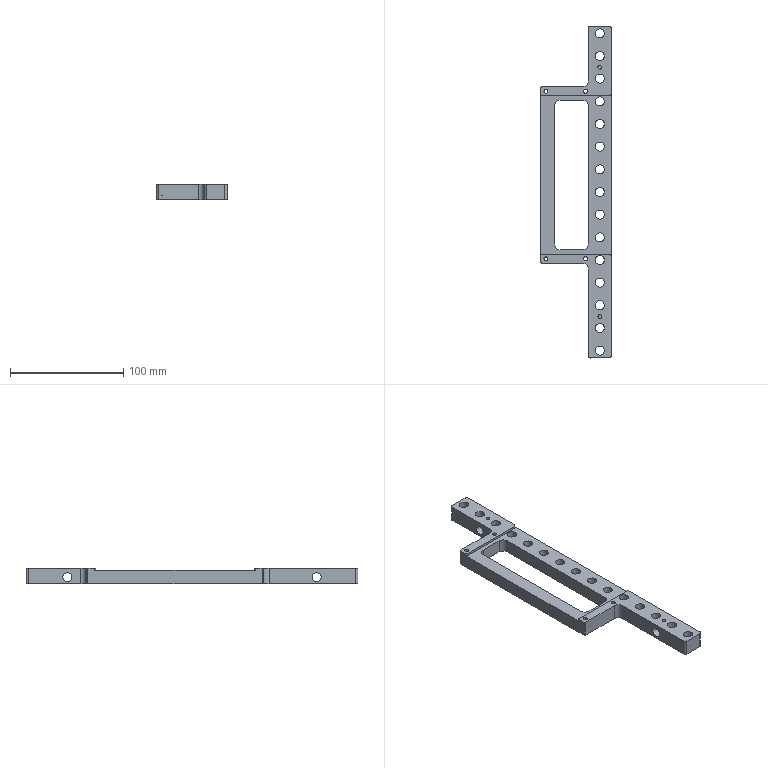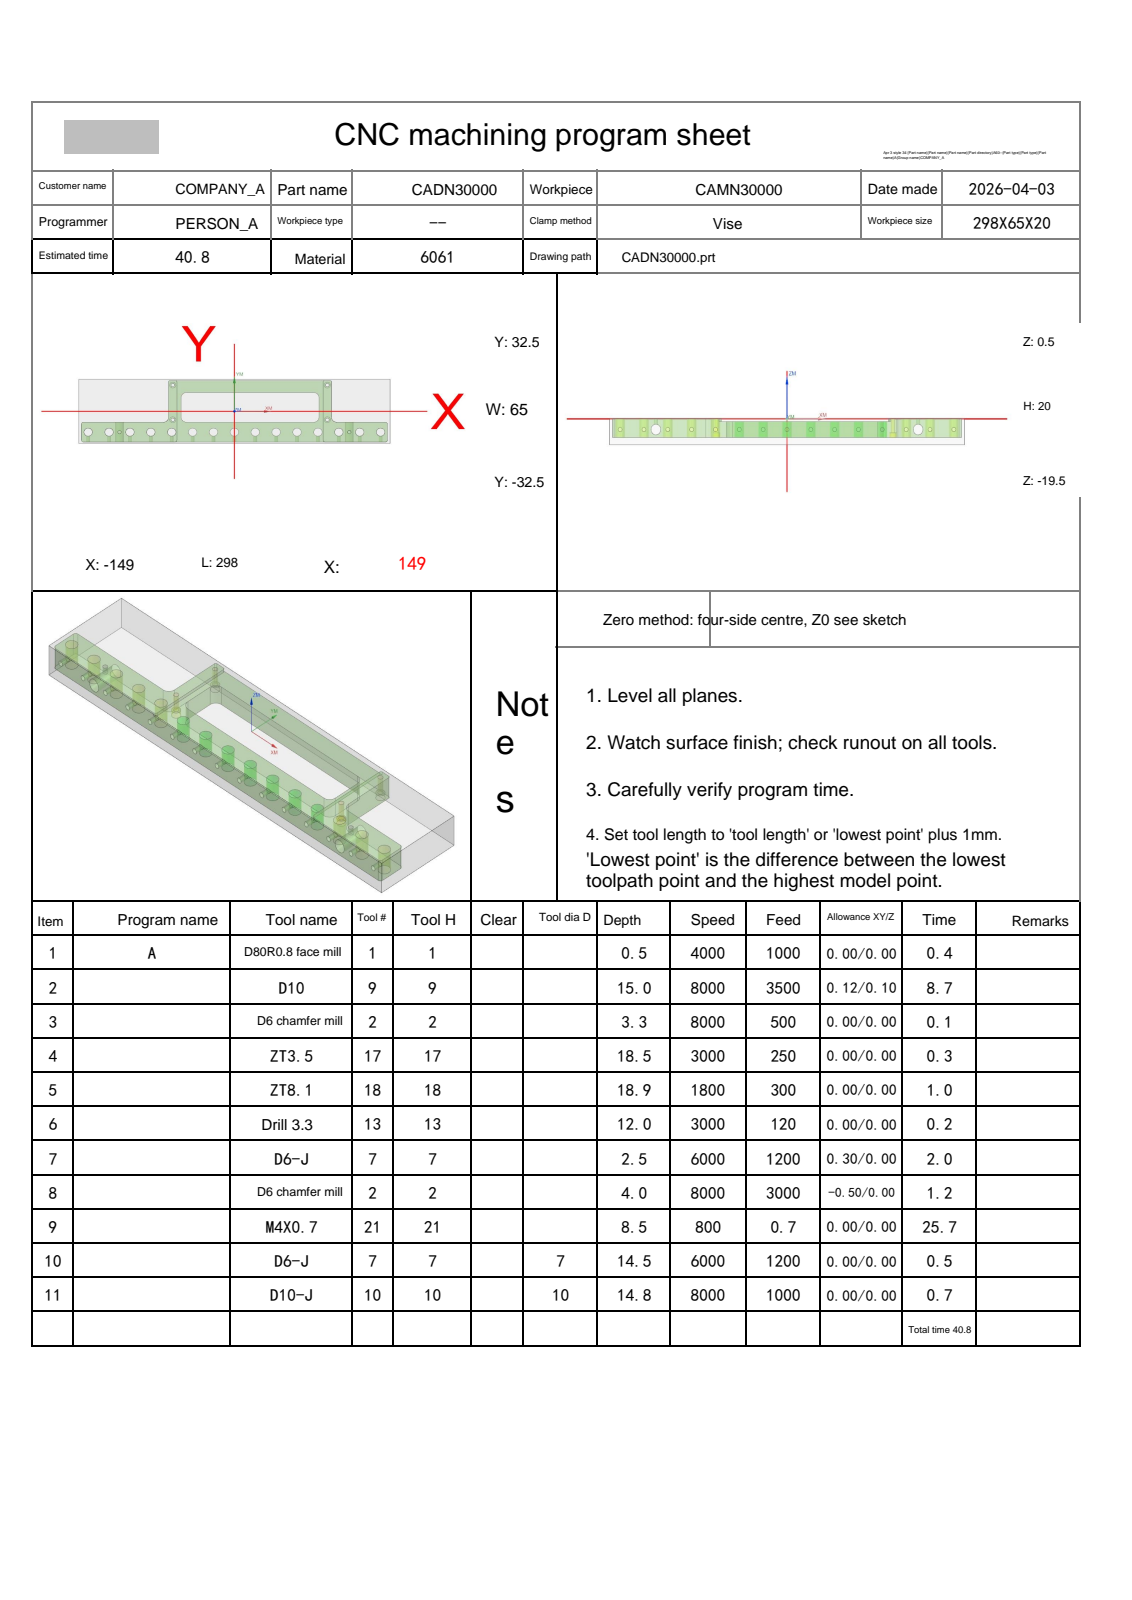NC program | NX | posted by the shop | part box 62 x 293 x 14 mm
Lines 1 to 35 of 5964:
%
O0001
(Machine time: 65.84 MIN)
(===Total Tool:9===)
(T1=D80R0.8 face mill D=80.  R=0.8  D-  H01 Z=-0.   )
(T9=D10     D=10.  R=0.   D-  H09 Z=-14.5 )
(T2=D6 chamfer mill   D=6.   R=0.   D-  H02 Z=-3.5  )
(T17=ZT3.5  D=3.5  DR_a=118 D-  H17 Z=-18.  )
(T18=ZT8.1  D=8.1  DR_a=118 D-  H18 Z=-18.43)
(T13=drill 3.3  D=3.3  DR_a=118 D-  H13 Z=-11.5 )
(T7=D6-J    D=6.   R=0.   D-  H07 Z=-14.  )
(T21=M4X0.7 D=3.3  DR_a=180 D-  H21 Z=-8.   )
(T10=D10-J  D=10.  R=0.   D10 H10 Z=-14.3 )
G80 G90 G17 G49 G40
G91 G28 Z0
M01
N1 T01 M06
(D80R0.8 face mill  D=80. R=0.8 H=01 ce=0.00 di=0.00)
G00 G90 G54 X-191.5 Y0.0 M03 S4000
G43 H01 Z20.
M08
Z2.
G01 Z0.0 F1000.
X-186.5
X186.5
X191.5
Z2.
G00 Z20.
G91 G28 Z0.0
M05
M09
G91 G28 Z0.0
M01